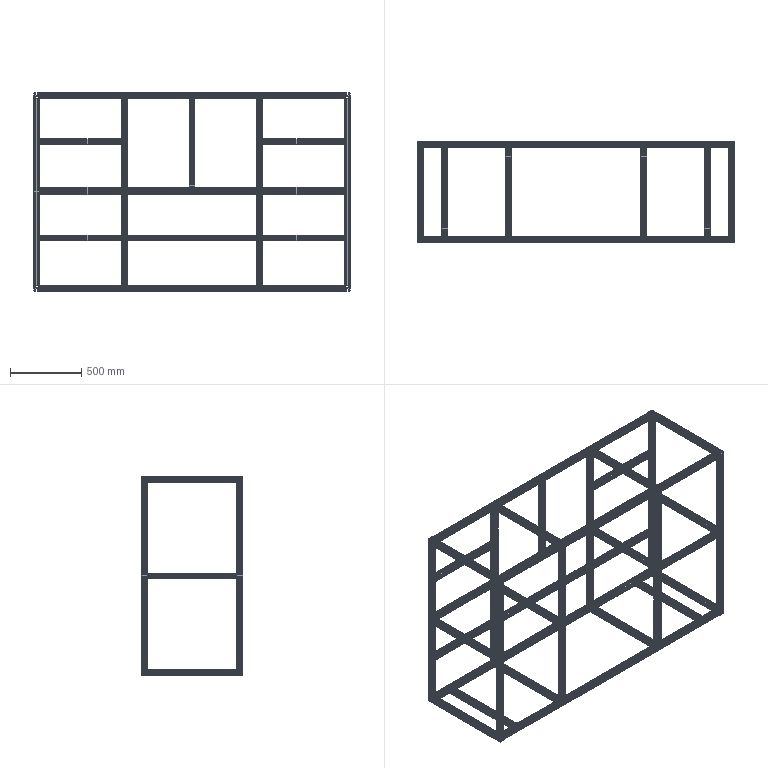Part | SolidWorks | features WeldCornerFeat 2, 3DProfileFeature 1, WeldMemberFeat 1, WeldmentFeature 1 | 38 solids | 3496 faces | volume 21852981 mm3 | plane 2964 | cylinder 532 | commonest cylinder face diameters 6 x304 9 x152 6.8 x76